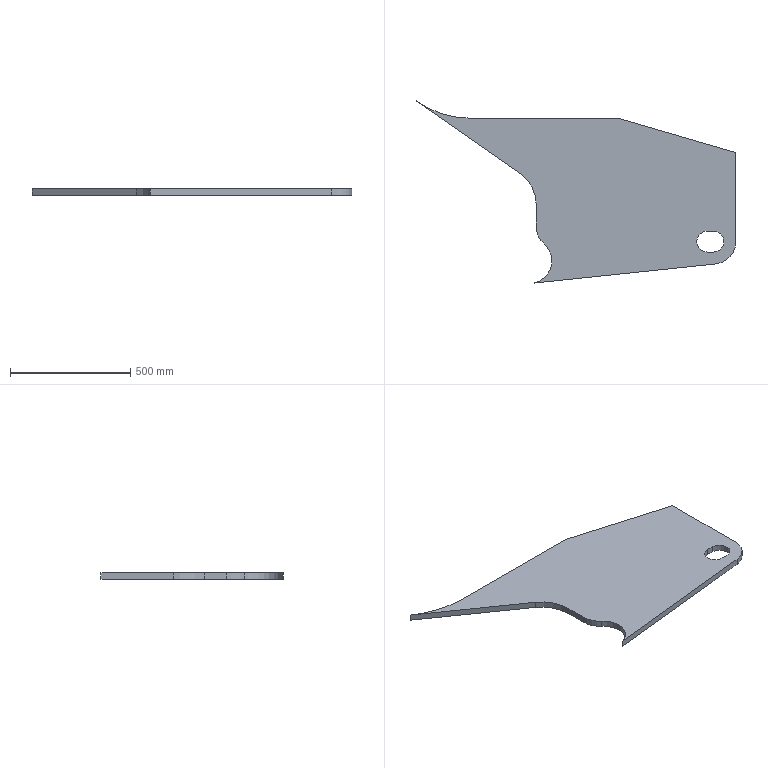Part | NX | features 底座(默认<按焊接>) 2 | 1 solid | 17 faces | box 1332 x 758.269 x 26 mm | volume 13979439 mm3 | plane 10 | cylinder 7 | commonest cylinder face diameters 87.28 x2 187.6 x2 200 x1 310 x1 800 x1
STEP:
#1=CARTESIAN_POINT('',(2693.125,23.856,-412.));
#2=VERTEX_POINT('',#1);
#3=CARTESIAN_POINT('',(3449.658,103.111,-412.));
#4=VERTEX_POINT('',#3);
#5=CARTESIAN_POINT('',(2789.761,33.98,-412.));
#6=DIRECTION('',(0.9946,0.1042,0.));
#7=VECTOR('',#6,1000.);
#8=LINE('',#5,#7);
#9=EDGE_CURVE('',#2,#4,#8,.T.);
#10=ORIENTED_EDGE('',*,*,#9,.T.);
#11=CARTESIAN_POINT('',(3449.658,103.111,-386.));
#12=VERTEX_POINT('',#11);
#13=CARTESIAN_POINT('',(3449.658,103.111,-386.));
#14=DIRECTION('',(0.,0.,-1.));
#15=VECTOR('',#14,1000.);
#16=LINE('',#13,#15);
#17=EDGE_CURVE('',#12,#4,#16,.T.);
#18=ORIENTED_EDGE('',*,*,#17,.F.);
#19=CARTESIAN_POINT('',(2693.125,23.856,-386.));
#20=VERTEX_POINT('',#19);
#21=CARTESIAN_POINT('',(2789.761,33.98,-386.));
#22=DIRECTION('',(0.9946,0.1042,0.));
#23=VECTOR('',#22,1000.);
#24=LINE('',#21,#23);
#25=EDGE_CURVE('',#20,#12,#24,.T.);
#26=ORIENTED_EDGE('',*,*,#25,.F.);
#27=CARTESIAN_POINT('',(2693.125,23.856,-386.));
#28=DIRECTION('',(0.,0.,-1.));
#29=VECTOR('',#28,1000.);
#30=LINE('',#27,#29);
#31=EDGE_CURVE('',#20,#2,#30,.T.);
#32=ORIENTED_EDGE('',*,*,#31,.T.);
#33=EDGE_LOOP('',(#10,#18,#26,#32));
#34=FACE_BOUND('',#33,.T.);
#35=CARTESIAN_POINT('',(2789.761,33.98,-386.));
#36=DIRECTION('',(0.1042,-0.9946,0.));
#37=DIRECTION('',(0.9946,0.1042,0.));
#38=AXIS2_PLACEMENT_3D('',#35,#36,#37);
#39=PLANE('',#38);
#40=ADVANCED_FACE('',(#34),#39,.T.);
#41=CARTESIAN_POINT('',(2735.88,185.836,-412.));
#42=VERTEX_POINT('',#41);
#43=CARTESIAN_POINT('',(2673.685,115.62,-412.));
#44=DIRECTION('',(0.,0.,1.));
#45=DIRECTION('',(1.,0.,0.));
#46=AXIS2_PLACEMENT_3D('',#43,#44,#45);
#47=CIRCLE('',#46,93.8);
#48=EDGE_CURVE('',#42,#2,#47,.F.);
#49=ORIENTED_EDGE('',*,*,#48,.T.);
#50=ORIENTED_EDGE('',*,*,#31,.F.);
#51=CARTESIAN_POINT('',(2735.88,185.836,-386.));
#52=VERTEX_POINT('',#51);
#53=CARTESIAN_POINT('',(2673.685,115.62,-386.));
#54=DIRECTION('',(0.,0.,1.));
#55=DIRECTION('',(1.,0.,0.));
#56=AXIS2_PLACEMENT_3D('',#53,#54,#55);
#57=CIRCLE('',#56,93.8);
#58=EDGE_CURVE('',#52,#20,#57,.F.);
#59=ORIENTED_EDGE('',*,*,#58,.F.);
#60=CARTESIAN_POINT('',(2735.88,185.836,-386.));
#61=DIRECTION('',(0.,0.,-1.));
#62=VECTOR('',#61,1000.);
#63=LINE('',#60,#62);
#64=EDGE_CURVE('',#52,#42,#63,.T.);
#65=ORIENTED_EDGE('',*,*,#64,.T.);
#66=EDGE_LOOP('',(#49,#50,#59,#65));
#67=FACE_BOUND('',#66,.T.);
#68=CARTESIAN_POINT('',(2673.685,115.62,-386.));
#69=DIRECTION('',(0.,0.,-1.));
#70=DIRECTION('',(1.,0.,0.));
#71=AXIS2_PLACEMENT_3D('',#68,#69,#70);
#72=CYLINDRICAL_SURFACE('',#71,93.8);
#73=ADVANCED_FACE('',(#67),#72,.F.);
#74=CARTESIAN_POINT('',(2702.185,260.693,-412.));
#75=VERTEX_POINT('',#74);
#76=CARTESIAN_POINT('',(2802.185,260.693,-412.));
#77=DIRECTION('',(0.,0.,1.));
#78=DIRECTION('',(1.,0.,0.));
#79=AXIS2_PLACEMENT_3D('',#76,#77,#78);
#80=CIRCLE('',#79,100.);
#81=EDGE_CURVE('',#75,#42,#80,.T.);
#82=ORIENTED_EDGE('',*,*,#81,.T.);
#83=ORIENTED_EDGE('',*,*,#64,.F.);
#84=CARTESIAN_POINT('',(2702.185,260.693,-386.));
#85=VERTEX_POINT('',#84);
#86=CARTESIAN_POINT('',(2802.185,260.693,-386.));
#87=DIRECTION('',(0.,0.,1.));
#88=DIRECTION('',(1.,0.,0.));
#89=AXIS2_PLACEMENT_3D('',#86,#87,#88);
#90=CIRCLE('',#89,100.);
#91=EDGE_CURVE('',#85,#52,#90,.T.);
#92=ORIENTED_EDGE('',*,*,#91,.F.);
#93=CARTESIAN_POINT('',(2702.185,260.693,-386.));
#94=DIRECTION('',(0.,0.,-1.));
#95=VECTOR('',#94,1000.);
#96=LINE('',#93,#95);
#97=EDGE_CURVE('',#85,#75,#96,.T.);
#98=ORIENTED_EDGE('',*,*,#97,.T.);
#99=EDGE_LOOP('',(#82,#83,#92,#98));
#100=FACE_BOUND('',#99,.T.);
#101=CARTESIAN_POINT('',(2802.185,260.693,-386.));
#102=DIRECTION('',(0.,0.,-1.));
#103=DIRECTION('',(1.,0.,0.));
#104=AXIS2_PLACEMENT_3D('',#101,#102,#103);
#105=CYLINDRICAL_SURFACE('',#104,100.);
#106=ADVANCED_FACE('',(#100),#105,.T.);
#107=CARTESIAN_POINT('',(2702.185,351.82,-412.));
#108=VERTEX_POINT('',#107);
#109=CARTESIAN_POINT('',(2702.185,-779.355,-412.));
#110=DIRECTION('',(0.,-1.,0.));
#111=VECTOR('',#110,1000.);
#112=LINE('',#109,#111);
#113=EDGE_CURVE('',#108,#75,#112,.T.);
#114=ORIENTED_EDGE('',*,*,#113,.T.);
#115=ORIENTED_EDGE('',*,*,#97,.F.);
#116=CARTESIAN_POINT('',(2702.185,351.82,-386.));
#117=VERTEX_POINT('',#116);
#118=CARTESIAN_POINT('',(2702.185,-779.355,-386.));
#119=DIRECTION('',(0.,-1.,0.));
#120=VECTOR('',#119,1000.);
#121=LINE('',#118,#120);
#122=EDGE_CURVE('',#117,#85,#121,.T.);
#123=ORIENTED_EDGE('',*,*,#122,.F.);
#124=CARTESIAN_POINT('',(2702.185,351.82,-386.));
#125=DIRECTION('',(0.,0.,-1.));
#126=VECTOR('',#125,1000.);
#127=LINE('',#124,#126);
#128=EDGE_CURVE('',#117,#108,#127,.T.);
#129=ORIENTED_EDGE('',*,*,#128,.T.);
#130=EDGE_LOOP('',(#114,#115,#123,#129));
#131=FACE_BOUND('',#130,.T.);
#132=CARTESIAN_POINT('',(2702.185,-779.355,-386.));
#133=DIRECTION('',(-1.,0.,0.));
#134=DIRECTION('',(0.,0.,-1.));
#135=AXIS2_PLACEMENT_3D('',#132,#133,#134);
#136=PLANE('',#135);
#137=ADVANCED_FACE('',(#131),#136,.T.);
#138=CARTESIAN_POINT('',(2635.971,478.871,-412.));
#139=VERTEX_POINT('',#138);
#140=CARTESIAN_POINT('',(2547.185,351.82,-412.));
#141=DIRECTION('',(0.,0.,1.));
#142=DIRECTION('',(1.,0.,0.));
#143=AXIS2_PLACEMENT_3D('',#140,#141,#142);
#144=CIRCLE('',#143,155.);
#145=EDGE_CURVE('',#139,#108,#144,.F.);
#146=ORIENTED_EDGE('',*,*,#145,.T.);
#147=ORIENTED_EDGE('',*,*,#128,.F.);
#148=CARTESIAN_POINT('',(2635.971,478.871,-386.));
#149=VERTEX_POINT('',#148);
#150=CARTESIAN_POINT('',(2547.185,351.82,-386.));
#151=DIRECTION('',(0.,0.,1.));
#152=DIRECTION('',(1.,0.,0.));
#153=AXIS2_PLACEMENT_3D('',#150,#151,#152);
#154=CIRCLE('',#153,155.);
#155=EDGE_CURVE('',#149,#117,#154,.F.);
#156=ORIENTED_EDGE('',*,*,#155,.F.);
#157=CARTESIAN_POINT('',(2635.971,478.871,-386.));
#158=DIRECTION('',(0.,0.,-1.));
#159=VECTOR('',#158,1000.);
#160=LINE('',#157,#159);
#161=EDGE_CURVE('',#149,#139,#160,.T.);
#162=ORIENTED_EDGE('',*,*,#161,.T.);
#163=EDGE_LOOP('',(#146,#147,#156,#162));
#164=FACE_BOUND('',#163,.T.);
#165=CARTESIAN_POINT('',(2547.185,351.82,-386.));
#166=DIRECTION('',(0.,0.,-1.));
#167=DIRECTION('',(1.,0.,0.));
#168=AXIS2_PLACEMENT_3D('',#165,#166,#167);
#169=CYLINDRICAL_SURFACE('',#168,155.);
#170=ADVANCED_FACE('',(#164),#169,.F.);
#171=CARTESIAN_POINT('',(2202.02,782.126,-412.));
#172=VERTEX_POINT('',#171);
#173=CARTESIAN_POINT('',(3387.32,-46.187,-412.));
#174=DIRECTION('',(0.8197,-0.5728,0.));
#175=VECTOR('',#174,1000.);
#176=LINE('',#173,#175);
#177=EDGE_CURVE('',#172,#139,#176,.T.);
#178=ORIENTED_EDGE('',*,*,#177,.T.);
#179=ORIENTED_EDGE('',*,*,#161,.F.);
#180=CARTESIAN_POINT('',(2202.02,782.126,-386.));
#181=VERTEX_POINT('',#180);
#182=CARTESIAN_POINT('',(3387.32,-46.187,-386.));
#183=DIRECTION('',(0.8197,-0.5728,0.));
#184=VECTOR('',#183,1000.);
#185=LINE('',#182,#184);
#186=EDGE_CURVE('',#181,#149,#185,.T.);
#187=ORIENTED_EDGE('',*,*,#186,.F.);
#188=CARTESIAN_POINT('',(2202.02,782.126,-386.));
#189=DIRECTION('',(0.,0.,-1.));
#190=VECTOR('',#189,1000.);
#191=LINE('',#188,#190);
#192=EDGE_CURVE('',#181,#172,#191,.T.);
#193=ORIENTED_EDGE('',*,*,#192,.T.);
#194=EDGE_LOOP('',(#178,#179,#187,#193));
#195=FACE_BOUND('',#194,.T.);
#196=CARTESIAN_POINT('',(3387.32,-46.187,-386.));
#197=DIRECTION('',(-0.5728,-0.8197,0.));
#198=DIRECTION('',(0.8197,-0.5728,0.));
#199=AXIS2_PLACEMENT_3D('',#196,#197,#198);
#200=PLANE('',#199);
#201=ADVANCED_FACE('',(#195),#200,.T.);
#202=CARTESIAN_POINT('',(2431.145,710.,-412.));
#203=VERTEX_POINT('',#202);
#204=CARTESIAN_POINT('',(2431.145,1110.,-412.));
#205=DIRECTION('',(0.,0.,1.));
#206=DIRECTION('',(1.,0.,0.));
#207=AXIS2_PLACEMENT_3D('',#204,#205,#206);
#208=CIRCLE('',#207,400.);
#209=EDGE_CURVE('',#172,#203,#208,.T.);
#210=ORIENTED_EDGE('',*,*,#209,.F.);
#211=ORIENTED_EDGE('',*,*,#192,.F.);
#212=CARTESIAN_POINT('',(2431.145,710.,-386.));
#213=VERTEX_POINT('',#212);
#214=CARTESIAN_POINT('',(2431.145,1110.,-386.));
#215=DIRECTION('',(0.,0.,1.));
#216=DIRECTION('',(1.,0.,0.));
#217=AXIS2_PLACEMENT_3D('',#214,#215,#216);
#218=CIRCLE('',#217,400.);
#219=EDGE_CURVE('',#181,#213,#218,.T.);
#220=ORIENTED_EDGE('',*,*,#219,.T.);
#221=CARTESIAN_POINT('',(2431.145,710.,-386.));
#222=DIRECTION('',(0.,0.,-1.));
#223=VECTOR('',#222,1000.);
#224=LINE('',#221,#223);
#225=EDGE_CURVE('',#213,#203,#224,.T.);
#226=ORIENTED_EDGE('',*,*,#225,.T.);
#227=EDGE_LOOP('',(#210,#211,#220,#226));
#228=FACE_BOUND('',#227,.T.);
#229=CARTESIAN_POINT('',(2431.145,1110.,-386.));
#230=DIRECTION('',(0.,0.,-1.));
#231=DIRECTION('',(1.,0.,0.));
#232=AXIS2_PLACEMENT_3D('',#229,#230,#231);
#233=CYLINDRICAL_SURFACE('',#232,400.);
#234=ADVANCED_FACE('',(#228),#233,.F.);
#235=CARTESIAN_POINT('',(3044.885,710.,-412.));
#236=VERTEX_POINT('',#235);
#237=CARTESIAN_POINT('',(2874.966,710.,-412.));
#238=DIRECTION('',(-1.,0.,0.));
#239=VECTOR('',#238,1000.);
#240=LINE('',#237,#239);
#241=EDGE_CURVE('',#236,#203,#240,.T.);
#242=ORIENTED_EDGE('',*,*,#241,.T.);
#243=ORIENTED_EDGE('',*,*,#225,.F.);
#244=CARTESIAN_POINT('',(3044.885,710.,-386.));
#245=VERTEX_POINT('',#244);
#246=CARTESIAN_POINT('',(2874.966,710.,-386.));
#247=DIRECTION('',(-1.,0.,0.));
#248=VECTOR('',#247,1000.);
#249=LINE('',#246,#248);
#250=EDGE_CURVE('',#245,#213,#249,.T.);
#251=ORIENTED_EDGE('',*,*,#250,.F.);
#252=CARTESIAN_POINT('',(3044.885,710.,-386.));
#253=DIRECTION('',(0.,0.,-1.));
#254=VECTOR('',#253,1000.);
#255=LINE('',#252,#254);
#256=EDGE_CURVE('',#245,#236,#255,.T.);
#257=ORIENTED_EDGE('',*,*,#256,.T.);
#258=EDGE_LOOP('',(#242,#243,#251,#257));
#259=FACE_BOUND('',#258,.T.);
#260=CARTESIAN_POINT('',(2874.966,710.,-386.));
#261=DIRECTION('',(0.,1.,0.));
#262=DIRECTION('',(0.,0.,-1.));
#263=AXIS2_PLACEMENT_3D('',#260,#261,#262);
#264=PLANE('',#263);
#265=ADVANCED_FACE('',(#259),#264,.T.);
#266=CARTESIAN_POINT('',(3533.685,567.32,-412.));
#267=VERTEX_POINT('',#266);
#268=CARTESIAN_POINT('',(3288.914,638.768,-412.));
#269=DIRECTION('',(-0.9599,0.2802,0.));
#270=VECTOR('',#269,1000.);
#271=LINE('',#268,#270);
#272=EDGE_CURVE('',#267,#236,#271,.T.);
#273=ORIENTED_EDGE('',*,*,#272,.T.);
#274=ORIENTED_EDGE('',*,*,#256,.F.);
#275=CARTESIAN_POINT('',(3533.685,567.32,-386.));
#276=VERTEX_POINT('',#275);
#277=CARTESIAN_POINT('',(3288.914,638.768,-386.));
#278=DIRECTION('',(-0.9599,0.2802,0.));
#279=VECTOR('',#278,1000.);
#280=LINE('',#277,#279);
#281=EDGE_CURVE('',#276,#245,#280,.T.);
#282=ORIENTED_EDGE('',*,*,#281,.F.);
#283=CARTESIAN_POINT('',(3533.685,567.32,-386.));
#284=DIRECTION('',(0.,0.,-1.));
#285=VECTOR('',#284,1000.);
#286=LINE('',#283,#285);
#287=EDGE_CURVE('',#276,#267,#286,.T.);
#288=ORIENTED_EDGE('',*,*,#287,.T.);
#289=EDGE_LOOP('',(#273,#274,#282,#288));
#290=FACE_BOUND('',#289,.T.);
#291=CARTESIAN_POINT('',(3288.914,638.768,-386.));
#292=DIRECTION('',(0.2802,0.9599,0.));
#293=DIRECTION('',(-0.9599,0.2802,0.));
#294=AXIS2_PLACEMENT_3D('',#291,#292,#293);
#295=PLANE('',#294);
#296=ADVANCED_FACE('',(#290),#295,.T.);
#297=CARTESIAN_POINT('',(3533.685,196.4,-412.));
#298=VERTEX_POINT('',#297);
#299=CARTESIAN_POINT('',(3533.685,-779.355,-412.));
#300=DIRECTION('',(0.,-1.,0.));
#301=VECTOR('',#300,1000.);
#302=LINE('',#299,#301);
#303=EDGE_CURVE('',#267,#298,#302,.T.);
#304=ORIENTED_EDGE('',*,*,#303,.F.);
#305=ORIENTED_EDGE('',*,*,#287,.F.);
#306=CARTESIAN_POINT('',(3533.685,196.4,-386.));
#307=VERTEX_POINT('',#306);
#308=CARTESIAN_POINT('',(3533.685,-779.355,-386.));
#309=DIRECTION('',(0.,-1.,0.));
#310=VECTOR('',#309,1000.);
#311=LINE('',#308,#310);
#312=EDGE_CURVE('',#276,#307,#311,.T.);
#313=ORIENTED_EDGE('',*,*,#312,.T.);
#314=CARTESIAN_POINT('',(3533.685,196.4,-386.));
#315=DIRECTION('',(0.,0.,-1.));
#316=VECTOR('',#315,1000.);
#317=LINE('',#314,#316);
#318=EDGE_CURVE('',#307,#298,#317,.T.);
#319=ORIENTED_EDGE('',*,*,#318,.T.);
#320=EDGE_LOOP('',(#304,#305,#313,#319));
#321=FACE_BOUND('',#320,.T.);
#322=CARTESIAN_POINT('',(3533.685,-779.355,-386.));
#323=DIRECTION('',(-1.,0.,0.));
#324=DIRECTION('',(0.,0.,-1.));
#325=AXIS2_PLACEMENT_3D('',#322,#323,#324);
#326=PLANE('',#325);
#327=ADVANCED_FACE('',(#321),#326,.F.);
#328=CARTESIAN_POINT('',(3439.885,196.4,-412.));
#329=DIRECTION('',(0.,0.,1.));
#330=DIRECTION('',(1.,0.,0.));
#331=AXIS2_PLACEMENT_3D('',#328,#329,#330);
#332=CIRCLE('',#331,93.8);
#333=EDGE_CURVE('',#4,#298,#332,.T.);
#334=ORIENTED_EDGE('',*,*,#333,.T.);
#335=ORIENTED_EDGE('',*,*,#318,.F.);
#336=CARTESIAN_POINT('',(3439.885,196.4,-386.));
#337=DIRECTION('',(0.,0.,1.));
#338=DIRECTION('',(1.,0.,0.));
#339=AXIS2_PLACEMENT_3D('',#336,#337,#338);
#340=CIRCLE('',#339,93.8);
#341=EDGE_CURVE('',#12,#307,#340,.T.);
#342=ORIENTED_EDGE('',*,*,#341,.F.);
#343=ORIENTED_EDGE('',*,*,#17,.T.);
#344=EDGE_LOOP('',(#334,#335,#342,#343));
#345=FACE_BOUND('',#344,.T.);
#346=CARTESIAN_POINT('',(3439.885,196.4,-386.));
#347=DIRECTION('',(0.,0.,-1.));
#348=DIRECTION('',(1.,0.,0.));
#349=AXIS2_PLACEMENT_3D('',#346,#347,#348);
#350=CYLINDRICAL_SURFACE('',#349,93.8);
#351=ADVANCED_FACE('',(#345),#350,.T.);
#352=CARTESIAN_POINT('',(3439.885,240.04,-386.));
#353=VERTEX_POINT('',#352);
#354=CARTESIAN_POINT('',(3414.885,240.04,-386.));
#355=VERTEX_POINT('',#354);
#356=CARTESIAN_POINT('',(2874.966,240.04,-386.));
#357=DIRECTION('',(-1.,0.,0.));
#358=VECTOR('',#357,1000.);
#359=LINE('',#356,#358);
#360=EDGE_CURVE('',#353,#355,#359,.T.);
#361=ORIENTED_EDGE('',*,*,#360,.F.);
#362=CARTESIAN_POINT('',(3439.885,152.76,-386.));
#363=VERTEX_POINT('',#362);
#364=CARTESIAN_POINT('',(3439.885,196.4,-386.));
#365=DIRECTION('',(0.,0.,1.));
#366=DIRECTION('',(1.,0.,0.));
#367=AXIS2_PLACEMENT_3D('',#364,#365,#366);
#368=CIRCLE('',#367,43.64);
#369=EDGE_CURVE('',#363,#353,#368,.T.);
#370=ORIENTED_EDGE('',*,*,#369,.F.);
#371=CARTESIAN_POINT('',(3414.885,152.76,-386.));
#372=VERTEX_POINT('',#371);
#373=CARTESIAN_POINT('',(2874.966,152.76,-386.));
#374=DIRECTION('',(1.,0.,0.));
#375=VECTOR('',#374,1000.);
#376=LINE('',#373,#375);
#377=EDGE_CURVE('',#372,#363,#376,.T.);
#378=ORIENTED_EDGE('',*,*,#377,.F.);
#379=CARTESIAN_POINT('',(3414.885,196.4,-386.));
#380=DIRECTION('',(0.,0.,1.));
#381=DIRECTION('',(1.,0.,0.));
#382=AXIS2_PLACEMENT_3D('',#379,#380,#381);
#383=CIRCLE('',#382,43.64);
#384=EDGE_CURVE('',#355,#372,#383,.T.);
#385=ORIENTED_EDGE('',*,*,#384,.F.);
#386=EDGE_LOOP('',(#361,#370,#378,#385));
#387=FACE_BOUND('',#386,.T.);
#388=ORIENTED_EDGE('',*,*,#25,.T.);
#389=ORIENTED_EDGE('',*,*,#341,.T.);
#390=ORIENTED_EDGE('',*,*,#312,.F.);
#391=ORIENTED_EDGE('',*,*,#281,.T.);
#392=ORIENTED_EDGE('',*,*,#250,.T.);
#393=ORIENTED_EDGE('',*,*,#219,.F.);
#394=ORIENTED_EDGE('',*,*,#186,.T.);
#395=ORIENTED_EDGE('',*,*,#155,.T.);
#396=ORIENTED_EDGE('',*,*,#122,.T.);
#397=ORIENTED_EDGE('',*,*,#91,.T.);
#398=ORIENTED_EDGE('',*,*,#58,.T.);
#399=EDGE_LOOP('',(#388,#389,#390,#391,#392,#393,#394,#395,#396,#397,#398));
#400=FACE_BOUND('',#399,.T.);
#401=CARTESIAN_POINT('',(2874.966,-779.355,-386.));
#402=DIRECTION('',(0.,0.,-1.));
#403=DIRECTION('',(1.,0.,0.));
#404=AXIS2_PLACEMENT_3D('',#401,#402,#403);
#405=PLANE('',#404);
#406=ADVANCED_FACE('',(#387,#400),#405,.F.);
#407=CARTESIAN_POINT('',(3414.885,240.04,-412.));
#408=VERTEX_POINT('',#407);
#409=CARTESIAN_POINT('',(3414.885,152.76,-412.));
#410=VERTEX_POINT('',#409);
#411=CARTESIAN_POINT('',(3414.885,196.4,-412.));
#412=DIRECTION('',(0.,0.,1.));
#413=DIRECTION('',(1.,0.,0.));
#414=AXIS2_PLACEMENT_3D('',#411,#412,#413);
#415=CIRCLE('',#414,43.64);
#416=EDGE_CURVE('',#408,#410,#415,.T.);
#417=ORIENTED_EDGE('',*,*,#416,.T.);
#418=CARTESIAN_POINT('',(3439.885,152.76,-412.));
#419=VERTEX_POINT('',#418);
#420=CARTESIAN_POINT('',(2874.966,152.76,-412.));
#421=DIRECTION('',(1.,0.,0.));
#422=VECTOR('',#421,1000.);
#423=LINE('',#420,#422);
#424=EDGE_CURVE('',#410,#419,#423,.T.);
#425=ORIENTED_EDGE('',*,*,#424,.T.);
#426=CARTESIAN_POINT('',(3439.885,240.04,-412.));
#427=VERTEX_POINT('',#426);
#428=CARTESIAN_POINT('',(3439.885,196.4,-412.));
#429=DIRECTION('',(0.,0.,1.));
#430=DIRECTION('',(1.,0.,0.));
#431=AXIS2_PLACEMENT_3D('',#428,#429,#430);
#432=CIRCLE('',#431,43.64);
#433=EDGE_CURVE('',#419,#427,#432,.T.);
#434=ORIENTED_EDGE('',*,*,#433,.T.);
#435=CARTESIAN_POINT('',(2874.966,240.04,-412.));
#436=DIRECTION('',(-1.,0.,0.));
#437=VECTOR('',#436,1000.);
#438=LINE('',#435,#437);
#439=EDGE_CURVE('',#427,#408,#438,.T.);
#440=ORIENTED_EDGE('',*,*,#439,.T.);
#441=EDGE_LOOP('',(#417,#425,#434,#440));
#442=FACE_BOUND('',#441,.T.);
#443=ORIENTED_EDGE('',*,*,#9,.F.);
#444=ORIENTED_EDGE('',*,*,#48,.F.);
#445=ORIENTED_EDGE('',*,*,#81,.F.);
#446=ORIENTED_EDGE('',*,*,#113,.F.);
#447=ORIENTED_EDGE('',*,*,#145,.F.);
#448=ORIENTED_EDGE('',*,*,#177,.F.);
#449=ORIENTED_EDGE('',*,*,#209,.T.);
#450=ORIENTED_EDGE('',*,*,#241,.F.);
#451=ORIENTED_EDGE('',*,*,#272,.F.);
#452=ORIENTED_EDGE('',*,*,#303,.T.);
#453=ORIENTED_EDGE('',*,*,#333,.F.);
#454=EDGE_LOOP('',(#443,#444,#445,#446,#447,#448,#449,#450,#451,#452,#453));
#455=FACE_BOUND('',#454,.T.);
#456=CARTESIAN_POINT('',(2874.966,-779.355,-412.));
#457=DIRECTION('',(0.,0.,-1.));
#458=DIRECTION('',(1.,0.,0.));
#459=AXIS2_PLACEMENT_3D('',#456,#457,#458);
#460=PLANE('',#459);
#461=ADVANCED_FACE('',(#442,#455),#460,.T.);
#462=CARTESIAN_POINT('',(3414.885,240.04,-26.));
#463=DIRECTION('',(0.,0.,-1.));
#464=VECTOR('',#463,1000.);
#465=LINE('',#462,#464);
#466=EDGE_CURVE('',#355,#408,#465,.T.);
#467=ORIENTED_EDGE('',*,*,#466,.F.);
#468=ORIENTED_EDGE('',*,*,#384,.T.);
#469=CARTESIAN_POINT('',(3414.885,152.76,-26.));
#470=DIRECTION('',(0.,0.,-1.));
#471=VECTOR('',#470,1000.);
#472=LINE('',#469,#471);
#473=EDGE_CURVE('',#372,#410,#472,.T.);
#474=ORIENTED_EDGE('',*,*,#473,.T.);
#475=ORIENTED_EDGE('',*,*,#416,.F.);
#476=EDGE_LOOP('',(#467,#468,#474,#475));
#477=FACE_BOUND('',#476,.T.);
#478=CARTESIAN_POINT('',(3414.885,196.4,-26.));
#479=DIRECTION('',(0.,0.,-1.));
#480=DIRECTION('',(1.,0.,0.));
#481=AXIS2_PLACEMENT_3D('',#478,#479,#480);
#482=CYLINDRICAL_SURFACE('',#481,43.64);
#483=ADVANCED_FACE('',(#477),#482,.F.);
#484=CARTESIAN_POINT('',(3439.885,240.04,-26.));
#485=DIRECTION('',(0.,0.,-1.));
#486=VECTOR('',#485,1000.);
#487=LINE('',#484,#486);
#488=EDGE_CURVE('',#353,#427,#487,.T.);
#489=ORIENTED_EDGE('',*,*,#488,.F.);
#490=ORIENTED_EDGE('',*,*,#360,.T.);
#491=ORIENTED_EDGE('',*,*,#466,.T.);
#492=ORIENTED_EDGE('',*,*,#439,.F.);
#493=EDGE_LOOP('',(#489,#490,#491,#492));
#494=FACE_BOUND('',#493,.T.);
#495=CARTESIAN_POINT('',(3414.885,240.04,-26.));
#496=DIRECTION('',(0.,1.,0.));
#497=DIRECTION('',(0.,0.,-1.));
#498=AXIS2_PLACEMENT_3D('',#495,#496,#497);
#499=PLANE('',#498);
#500=ADVANCED_FACE('',(#494),#499,.F.);
#501=CARTESIAN_POINT('',(3439.885,152.76,-26.));
#502=DIRECTION('',(0.,0.,-1.));
#503=VECTOR('',#502,1000.);
#504=LINE('',#501,#503);
#505=EDGE_CURVE('',#363,#419,#504,.T.);
#506=ORIENTED_EDGE('',*,*,#505,.F.);
#507=ORIENTED_EDGE('',*,*,#369,.T.);
#508=ORIENTED_EDGE('',*,*,#488,.T.);
#509=ORIENTED_EDGE('',*,*,#433,.F.);
#510=EDGE_LOOP('',(#506,#507,#508,#509));
#511=FACE_BOUND('',#510,.T.);
#512=CARTESIAN_POINT('',(3439.885,196.4,-26.));
#513=DIRECTION('',(0.,0.,-1.));
#514=DIRECTION('',(1.,0.,0.));
#515=AXIS2_PLACEMENT_3D('',#512,#513,#514);
#516=CYLINDRICAL_SURFACE('',#515,43.64);
#517=ADVANCED_FACE('',(#511),#516,.F.);
#518=ORIENTED_EDGE('',*,*,#473,.F.);
#519=ORIENTED_EDGE('',*,*,#377,.T.);
#520=ORIENTED_EDGE('',*,*,#505,.T.);
#521=ORIENTED_EDGE('',*,*,#424,.F.);
#522=EDGE_LOOP('',(#518,#519,#520,#521));
#523=FACE_BOUND('',#522,.T.);
#524=CARTESIAN_POINT('',(3414.885,152.76,-26.));
#525=DIRECTION('',(0.,-1.,0.));
#526=DIRECTION('',(0.,0.,1.));
#527=AXIS2_PLACEMENT_3D('',#524,#525,#526);
#528=PLANE('',#527);
#529=ADVANCED_FACE('',(#523),#528,.F.);
#530=CLOSED_SHELL('',(#40,#73,#106,#137,#170,#201,#234,#265,#296,#327,#351,#406,#461,#483,#500,#517,#529));
#531=MANIFOLD_SOLID_BREP('',#530);
#532=(LENGTH_UNIT()NAMED_UNIT(*)SI_UNIT(.MILLI.,.METRE.));
#533=UNCERTAINTY_MEASURE_WITH_UNIT(LENGTH_MEASURE(0.00001),#532,'','');
#534=(NAMED_UNIT(*)PLANE_ANGLE_UNIT()SI_UNIT($,.RADIAN.));
#535=(NAMED_UNIT(*)SI_UNIT($,.STERADIAN.)SOLID_ANGLE_UNIT());
#536=(GEOMETRIC_REPRESENTATION_CONTEXT(3)GLOBAL_UNCERTAINTY_ASSIGNED_CONTEXT((#533))GLOBAL_UNIT_ASSIGNED_CONTEXT((#532,#534,#535))REPRESENTATION_CONTEXT('',''));
#537=ADVANCED_BREP_SHAPE_REPRESENTATION('',(#531),#536);